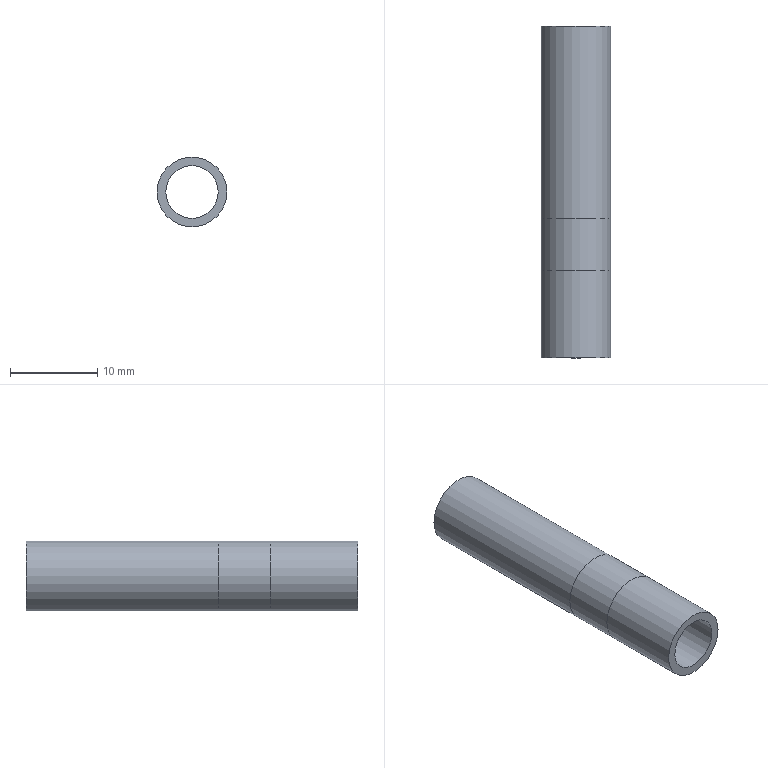Part | STEP file | 1-11.3 | 1 solid | 6 faces | box 8 x 38 x 8 mm | volume 835.664 mm3 | cylinder 4 | plane 2 | commonest cylinder face diameters 8 x3 6 x1
STEP:
#1=CARTESIAN_POINT('',(0.,0.,0.));
#2=DIRECTION('',(0.,0.,1.));
#3=DIRECTION('',(1.,0.,0.));
#4=AXIS2_PLACEMENT_3D('',#1,#2,#3);
#5=CARTESIAN_POINT('',(4.,19.,0.));
#6=VERTEX_POINT('',#5);
#7=CARTESIAN_POINT('',(0.,19.,0.));
#8=DIRECTION('',(0.,-1.,0.));
#9=DIRECTION('',(1.,0.,0.));
#10=AXIS2_PLACEMENT_3D('',#7,#8,#9);
#11=CIRCLE('',#10,4.);
#12=CARTESIAN_POINT('',(-1.072,19.,0.));
#13=DIRECTION('',(0.,-1.,0.));
#14=DIRECTION('',(1.,0.,0.));
#15=AXIS2_PLACEMENT_3D('',#12,#13,#14);
#16=PLANE('',#15);
#17=CARTESIAN_POINT('',(1.072,0.));
#18=DIRECTION('',(1.,0.));
#19=AXIS2_PLACEMENT_2D('',#17,#18);
#20=CIRCLE('',#19,4.);
#21=(GEOMETRIC_REPRESENTATION_CONTEXT(2)PARAMETRIC_REPRESENTATION_CONTEXT()REPRESENTATION_CONTEXT('',''));
#22=DEFINITIONAL_REPRESENTATION('',(#20),#21);
#23=PCURVE('',#16,#22);
#24=CARTESIAN_POINT('',(0.,19.,0.));
#25=DIRECTION('',(0.,-1.,0.));
#26=DIRECTION('',(1.,0.,0.));
#27=AXIS2_PLACEMENT_3D('',#24,#25,#26);
#28=CYLINDRICAL_SURFACE('',#27,4.);
#29=CARTESIAN_POINT('',(0.,0.));
#30=DIRECTION('',(1.,0.));
#31=VECTOR('',#30,1.);
#32=LINE('',#29,#31);
#33=(GEOMETRIC_REPRESENTATION_CONTEXT(2)PARAMETRIC_REPRESENTATION_CONTEXT()REPRESENTATION_CONTEXT('',''));
#34=DEFINITIONAL_REPRESENTATION('',(#32),#33);
#35=PCURVE('',#28,#34);
#36=SURFACE_CURVE('',#11,(#23,#35),.PCURVE_S1.);
#37=EDGE_CURVE('',#6,#6,#36,.T.);
#38=ORIENTED_EDGE('',*,*,#37,.T.);
#39=EDGE_LOOP('',(#38));
#40=FACE_BOUND('',#39,.F.);
#41=CARTESIAN_POINT('',(3.,19.,0.));
#42=VERTEX_POINT('',#41);
#43=CARTESIAN_POINT('',(0.,19.,0.));
#44=DIRECTION('',(0.,1.,0.));
#45=DIRECTION('',(1.,0.,0.));
#46=AXIS2_PLACEMENT_3D('',#43,#44,#45);
#47=CIRCLE('',#46,3.);
#48=CARTESIAN_POINT('',(4.072,0.));
#49=CARTESIAN_POINT('',(4.072,-5.196));
#50=CARTESIAN_POINT('',(-0.4282,-2.598));
#51=CARTESIAN_POINT('',(-4.928,0.));
#52=CARTESIAN_POINT('',(-0.4282,2.598));
#53=CARTESIAN_POINT('',(4.072,5.196));
#54=CARTESIAN_POINT('',(4.072,0.));
#55=(BOUNDED_CURVE()B_SPLINE_CURVE(2,(#48,#49,#50,#51,#52,#53,#54),.UNSPECIFIED.,.T.,.F.)B_SPLINE_CURVE_WITH_KNOTS((1,2,2,2,2,1),(-2.094,0.,2.094,4.189,6.283,8.378),.UNSPECIFIED.)CURVE()GEOMETRIC_REPRESENTATION_ITEM()RATIONAL_B_SPLINE_CURVE((1.,0.5,1.,0.5,1.,0.5,1.))REPRESENTATION_ITEM(''));
#56=(GEOMETRIC_REPRESENTATION_CONTEXT(2)PARAMETRIC_REPRESENTATION_CONTEXT()REPRESENTATION_CONTEXT('',''));
#57=DEFINITIONAL_REPRESENTATION('',(#55),#56);
#58=PCURVE('',#16,#57);
#59=CARTESIAN_POINT('',(0.,19.,0.));
#60=DIRECTION('',(0.,-1.,0.));
#61=DIRECTION('',(1.,0.,0.));
#62=AXIS2_PLACEMENT_3D('',#59,#60,#61);
#63=CYLINDRICAL_SURFACE('',#62,3.);
#64=CARTESIAN_POINT('',(6.283,0.));
#65=DIRECTION('',(-1.,0.));
#66=VECTOR('',#65,1.);
#67=LINE('',#64,#66);
#68=(GEOMETRIC_REPRESENTATION_CONTEXT(2)PARAMETRIC_REPRESENTATION_CONTEXT()REPRESENTATION_CONTEXT('',''));
#69=DEFINITIONAL_REPRESENTATION('',(#67),#68);
#70=PCURVE('',#63,#69);
#71=SURFACE_CURVE('',#47,(#58,#70),.PCURVE_S1.);
#72=EDGE_CURVE('',#42,#42,#71,.T.);
#73=ORIENTED_EDGE('',*,*,#72,.T.);
#74=EDGE_LOOP('',(#73));
#75=FACE_BOUND('',#74,.F.);
#76=ADVANCED_FACE('',(#40,#75),#16,.F.);
#77=CARTESIAN_POINT('',(4.,-19.,0.));
#78=VERTEX_POINT('',#77);
#79=CARTESIAN_POINT('',(0.,-19.,0.));
#80=DIRECTION('',(0.,-1.,0.));
#81=DIRECTION('',(1.,0.,0.));
#82=AXIS2_PLACEMENT_3D('',#79,#80,#81);
#83=CIRCLE('',#82,4.);
#84=CARTESIAN_POINT('',(-1.072,-19.,0.));
#85=DIRECTION('',(0.,-1.,0.));
#86=DIRECTION('',(1.,0.,0.));
#87=AXIS2_PLACEMENT_3D('',#84,#85,#86);
#88=PLANE('',#87);
#89=CARTESIAN_POINT('',(1.072,0.));
#90=DIRECTION('',(1.,0.));
#91=AXIS2_PLACEMENT_2D('',#89,#90);
#92=CIRCLE('',#91,4.);
#93=(GEOMETRIC_REPRESENTATION_CONTEXT(2)PARAMETRIC_REPRESENTATION_CONTEXT()REPRESENTATION_CONTEXT('',''));
#94=DEFINITIONAL_REPRESENTATION('',(#92),#93);
#95=PCURVE('',#88,#94);
#96=CARTESIAN_POINT('',(0.,-9.,0.));
#97=DIRECTION('',(0.,-1.,0.));
#98=DIRECTION('',(1.,0.,0.));
#99=AXIS2_PLACEMENT_3D('',#96,#97,#98);
#100=CYLINDRICAL_SURFACE('',#99,4.);
#101=CARTESIAN_POINT('',(0.,10.));
#102=DIRECTION('',(1.,0.));
#103=VECTOR('',#102,1.);
#104=LINE('',#101,#103);
#105=(GEOMETRIC_REPRESENTATION_CONTEXT(2)PARAMETRIC_REPRESENTATION_CONTEXT()REPRESENTATION_CONTEXT('',''));
#106=DEFINITIONAL_REPRESENTATION('',(#104),#105);
#107=PCURVE('',#100,#106);
#108=SURFACE_CURVE('',#83,(#95,#107),.PCURVE_S1.);
#109=EDGE_CURVE('',#78,#78,#108,.T.);
#110=ORIENTED_EDGE('',*,*,#109,.T.);
#111=EDGE_LOOP('',(#110));
#112=FACE_BOUND('',#111,.T.);
#113=CARTESIAN_POINT('',(3.,-19.,0.));
#114=VERTEX_POINT('',#113);
#115=CARTESIAN_POINT('',(0.,-19.,0.));
#116=DIRECTION('',(0.,1.,0.));
#117=DIRECTION('',(1.,0.,0.));
#118=AXIS2_PLACEMENT_3D('',#115,#116,#117);
#119=CIRCLE('',#118,3.);
#120=CARTESIAN_POINT('',(4.072,0.));
#121=CARTESIAN_POINT('',(4.072,-5.196));
#122=CARTESIAN_POINT('',(-0.4282,-2.598));
#123=CARTESIAN_POINT('',(-4.928,0.));
#124=CARTESIAN_POINT('',(-0.4282,2.598));
#125=CARTESIAN_POINT('',(4.072,5.196));
#126=CARTESIAN_POINT('',(4.072,0.));
#127=(BOUNDED_CURVE()B_SPLINE_CURVE(2,(#120,#121,#122,#123,#124,#125,#126),.UNSPECIFIED.,.T.,.F.)B_SPLINE_CURVE_WITH_KNOTS((1,2,2,2,2,1),(-2.094,0.,2.094,4.189,6.283,8.378),.UNSPECIFIED.)CURVE()GEOMETRIC_REPRESENTATION_ITEM()RATIONAL_B_SPLINE_CURVE((1.,0.5,1.,0.5,1.,0.5,1.))REPRESENTATION_ITEM(''));
#128=(GEOMETRIC_REPRESENTATION_CONTEXT(2)PARAMETRIC_REPRESENTATION_CONTEXT()REPRESENTATION_CONTEXT('',''));
#129=DEFINITIONAL_REPRESENTATION('',(#127),#128);
#130=PCURVE('',#88,#129);
#131=CARTESIAN_POINT('',(6.283,38.));
#132=DIRECTION('',(-1.,0.));
#133=VECTOR('',#132,1.);
#134=LINE('',#131,#133);
#135=(GEOMETRIC_REPRESENTATION_CONTEXT(2)PARAMETRIC_REPRESENTATION_CONTEXT()REPRESENTATION_CONTEXT('',''));
#136=DEFINITIONAL_REPRESENTATION('',(#134),#135);
#137=PCURVE('',#63,#136);
#138=SURFACE_CURVE('',#119,(#130,#137),.PCURVE_S1.);
#139=EDGE_CURVE('',#114,#114,#138,.T.);
#140=ORIENTED_EDGE('',*,*,#139,.T.);
#141=EDGE_LOOP('',(#140));
#142=FACE_BOUND('',#141,.T.);
#143=ADVANCED_FACE('',(#112,#142),#88,.T.);
#144=CARTESIAN_POINT('',(3.,19.,0.));
#145=DIRECTION('',(0.,-1.,0.));
#146=VECTOR('',#145,1.);
#147=LINE('',#144,#146);
#148=CARTESIAN_POINT('',(6.283,0.));
#149=DIRECTION('',(0.,1.));
#150=VECTOR('',#149,1.);
#151=LINE('',#148,#150);
#152=(GEOMETRIC_REPRESENTATION_CONTEXT(2)PARAMETRIC_REPRESENTATION_CONTEXT()REPRESENTATION_CONTEXT('',''));
#153=DEFINITIONAL_REPRESENTATION('',(#151),#152);
#154=PCURVE('',#63,#153);
#155=CARTESIAN_POINT('',(0.,0.));
#156=DIRECTION('',(0.,1.));
#157=VECTOR('',#156,1.);
#158=LINE('',#155,#157);
#159=(GEOMETRIC_REPRESENTATION_CONTEXT(2)PARAMETRIC_REPRESENTATION_CONTEXT()REPRESENTATION_CONTEXT('',''));
#160=DEFINITIONAL_REPRESENTATION('',(#158),#159);
#161=PCURVE('',#63,#160);
#162=SEAM_CURVE('',#147,(#154,#161),.PCURVE_S1.);
#163=EDGE_CURVE('',#42,#114,#162,.T.);
#164=ORIENTED_EDGE('',*,*,#163,.T.);
#165=ORIENTED_EDGE('',*,*,#139,.T.);
#166=ORIENTED_EDGE('',*,*,#163,.F.);
#167=ORIENTED_EDGE('',*,*,#72,.F.);
#168=EDGE_LOOP('',(#164,#165,#166,#167));
#169=FACE_BOUND('',#168,.F.);
#170=ADVANCED_FACE('',(#169),#63,.F.);
#171=ORIENTED_EDGE('',*,*,#109,.F.);
#172=CARTESIAN_POINT('',(4.,-9.,0.));
#173=VERTEX_POINT('',#172);
#174=CARTESIAN_POINT('',(4.,-9.,0.));
#175=DIRECTION('',(0.,-1.,0.));
#176=VECTOR('',#175,1.);
#177=LINE('',#174,#176);
#178=CARTESIAN_POINT('',(0.,0.));
#179=DIRECTION('',(0.,1.));
#180=VECTOR('',#179,1.);
#181=LINE('',#178,#180);
#182=(GEOMETRIC_REPRESENTATION_CONTEXT(2)PARAMETRIC_REPRESENTATION_CONTEXT()REPRESENTATION_CONTEXT('',''));
#183=DEFINITIONAL_REPRESENTATION('',(#181),#182);
#184=PCURVE('',#100,#183);
#185=CARTESIAN_POINT('',(6.283,0.));
#186=DIRECTION('',(0.,1.));
#187=VECTOR('',#186,1.);
#188=LINE('',#185,#187);
#189=(GEOMETRIC_REPRESENTATION_CONTEXT(2)PARAMETRIC_REPRESENTATION_CONTEXT()REPRESENTATION_CONTEXT('',''));
#190=DEFINITIONAL_REPRESENTATION('',(#188),#189);
#191=PCURVE('',#100,#190);
#192=SEAM_CURVE('',#177,(#184,#191),.PCURVE_S1.);
#193=EDGE_CURVE('',#173,#78,#192,.T.);
#194=ORIENTED_EDGE('',*,*,#193,.F.);
#195=CARTESIAN_POINT('',(0.,-9.,0.));
#196=DIRECTION('',(0.,-1.,0.));
#197=DIRECTION('',(1.,0.,0.));
#198=AXIS2_PLACEMENT_3D('',#195,#196,#197);
#199=CIRCLE('',#198,4.);
#200=CARTESIAN_POINT('',(0.,0.));
#201=DIRECTION('',(1.,0.));
#202=VECTOR('',#201,1.);
#203=LINE('',#200,#202);
#204=(GEOMETRIC_REPRESENTATION_CONTEXT(2)PARAMETRIC_REPRESENTATION_CONTEXT()REPRESENTATION_CONTEXT('',''));
#205=DEFINITIONAL_REPRESENTATION('',(#203),#204);
#206=PCURVE('',#100,#205);
#207=CARTESIAN_POINT('',(0.,19.,0.));
#208=DIRECTION('',(0.,-1.,0.));
#209=DIRECTION('',(1.,0.,0.));
#210=AXIS2_PLACEMENT_3D('',#207,#208,#209);
#211=CYLINDRICAL_SURFACE('',#210,4.);
#212=CARTESIAN_POINT('',(0.,28.));
#213=DIRECTION('',(1.,0.));
#214=VECTOR('',#213,1.);
#215=LINE('',#212,#214);
#216=(GEOMETRIC_REPRESENTATION_CONTEXT(2)PARAMETRIC_REPRESENTATION_CONTEXT()REPRESENTATION_CONTEXT('',''));
#217=DEFINITIONAL_REPRESENTATION('',(#215),#216);
#218=PCURVE('',#211,#217);
#219=SURFACE_CURVE('',#199,(#206,#218),.PCURVE_S1.);
#220=EDGE_CURVE('',#173,#173,#219,.T.);
#221=ORIENTED_EDGE('',*,*,#220,.T.);
#222=ORIENTED_EDGE('',*,*,#193,.T.);
#223=EDGE_LOOP('',(#171,#194,#221,#222));
#224=FACE_BOUND('',#223,.T.);
#225=ADVANCED_FACE('',(#224),#100,.T.);
#226=ORIENTED_EDGE('',*,*,#37,.T.);
#227=CARTESIAN_POINT('',(4.,-3.,0.));
#228=VERTEX_POINT('',#227);
#229=CARTESIAN_POINT('',(4.,19.,0.));
#230=DIRECTION('',(0.,-1.,0.));
#231=VECTOR('',#230,1.);
#232=LINE('',#229,#231);
#233=CARTESIAN_POINT('',(6.283,0.));
#234=DIRECTION('',(0.,1.));
#235=VECTOR('',#234,1.);
#236=LINE('',#233,#235);
#237=(GEOMETRIC_REPRESENTATION_CONTEXT(2)PARAMETRIC_REPRESENTATION_CONTEXT()REPRESENTATION_CONTEXT('',''));
#238=DEFINITIONAL_REPRESENTATION('',(#236),#237);
#239=PCURVE('',#28,#238);
#240=CARTESIAN_POINT('',(0.,0.));
#241=DIRECTION('',(0.,1.));
#242=VECTOR('',#241,1.);
#243=LINE('',#240,#242);
#244=(GEOMETRIC_REPRESENTATION_CONTEXT(2)PARAMETRIC_REPRESENTATION_CONTEXT()REPRESENTATION_CONTEXT('',''));
#245=DEFINITIONAL_REPRESENTATION('',(#243),#244);
#246=PCURVE('',#28,#245);
#247=SEAM_CURVE('',#232,(#239,#246),.PCURVE_S1.);
#248=EDGE_CURVE('',#6,#228,#247,.T.);
#249=ORIENTED_EDGE('',*,*,#248,.T.);
#250=CARTESIAN_POINT('',(0.,-3.,0.));
#251=DIRECTION('',(0.,-1.,0.));
#252=DIRECTION('',(1.,0.,0.));
#253=AXIS2_PLACEMENT_3D('',#250,#251,#252);
#254=CIRCLE('',#253,4.);
#255=CARTESIAN_POINT('',(0.,22.));
#256=DIRECTION('',(1.,0.));
#257=VECTOR('',#256,1.);
#258=LINE('',#255,#257);
#259=(GEOMETRIC_REPRESENTATION_CONTEXT(2)PARAMETRIC_REPRESENTATION_CONTEXT()REPRESENTATION_CONTEXT('',''));
#260=DEFINITIONAL_REPRESENTATION('',(#258),#259);
#261=PCURVE('',#28,#260);
#262=CARTESIAN_POINT('',(0.,22.));
#263=DIRECTION('',(1.,0.));
#264=VECTOR('',#263,1.);
#265=LINE('',#262,#264);
#266=(GEOMETRIC_REPRESENTATION_CONTEXT(2)PARAMETRIC_REPRESENTATION_CONTEXT()REPRESENTATION_CONTEXT('',''));
#267=DEFINITIONAL_REPRESENTATION('',(#265),#266);
#268=PCURVE('',#211,#267);
#269=SURFACE_CURVE('',#254,(#261,#268),.PCURVE_S1.);
#270=EDGE_CURVE('',#228,#228,#269,.T.);
#271=ORIENTED_EDGE('',*,*,#270,.F.);
#272=ORIENTED_EDGE('',*,*,#248,.F.);
#273=EDGE_LOOP('',(#226,#249,#271,#272));
#274=FACE_BOUND('',#273,.T.);
#275=ADVANCED_FACE('',(#274),#28,.T.);
#276=ORIENTED_EDGE('',*,*,#220,.F.);
#277=CARTESIAN_POINT('',(4.,-3.,0.));
#278=DIRECTION('',(0.,-1.,0.));
#279=VECTOR('',#278,1.);
#280=LINE('',#277,#279);
#281=CARTESIAN_POINT('',(0.,22.));
#282=DIRECTION('',(0.,1.));
#283=VECTOR('',#282,1.);
#284=LINE('',#281,#283);
#285=(GEOMETRIC_REPRESENTATION_CONTEXT(2)PARAMETRIC_REPRESENTATION_CONTEXT()REPRESENTATION_CONTEXT('',''));
#286=DEFINITIONAL_REPRESENTATION('',(#284),#285);
#287=PCURVE('',#211,#286);
#288=CARTESIAN_POINT('',(6.283,22.));
#289=DIRECTION('',(0.,1.));
#290=VECTOR('',#289,1.);
#291=LINE('',#288,#290);
#292=(GEOMETRIC_REPRESENTATION_CONTEXT(2)PARAMETRIC_REPRESENTATION_CONTEXT()REPRESENTATION_CONTEXT('',''));
#293=DEFINITIONAL_REPRESENTATION('',(#291),#292);
#294=PCURVE('',#211,#293);
#295=SEAM_CURVE('',#280,(#287,#294),.PCURVE_S1.);
#296=EDGE_CURVE('',#228,#173,#295,.T.);
#297=ORIENTED_EDGE('',*,*,#296,.F.);
#298=ORIENTED_EDGE('',*,*,#270,.T.);
#299=ORIENTED_EDGE('',*,*,#296,.T.);
#300=EDGE_LOOP('',(#276,#297,#298,#299));
#301=FACE_BOUND('',#300,.T.);
#302=ADVANCED_FACE('',(#301),#211,.T.);
#303=CLOSED_SHELL('',(#76,#143,#170,#225,#275,#302));
#304=MANIFOLD_SOLID_BREP('',#303);
#305=(LENGTH_UNIT()NAMED_UNIT(*)SI_UNIT(.MILLI.,.METRE.));
#306=UNCERTAINTY_MEASURE_WITH_UNIT(LENGTH_MEASURE(0.0000001),#305,'','');
#307=(NAMED_UNIT(*)PLANE_ANGLE_UNIT()SI_UNIT($,.RADIAN.));
#308=(NAMED_UNIT(*)SI_UNIT($,.STERADIAN.)SOLID_ANGLE_UNIT());
#309=(GEOMETRIC_REPRESENTATION_CONTEXT(3)GLOBAL_UNCERTAINTY_ASSIGNED_CONTEXT((#306))GLOBAL_UNIT_ASSIGNED_CONTEXT((#305,#307,#308))REPRESENTATION_CONTEXT('',''));
#310=ADVANCED_BREP_SHAPE_REPRESENTATION('',(#4,#304),#309);